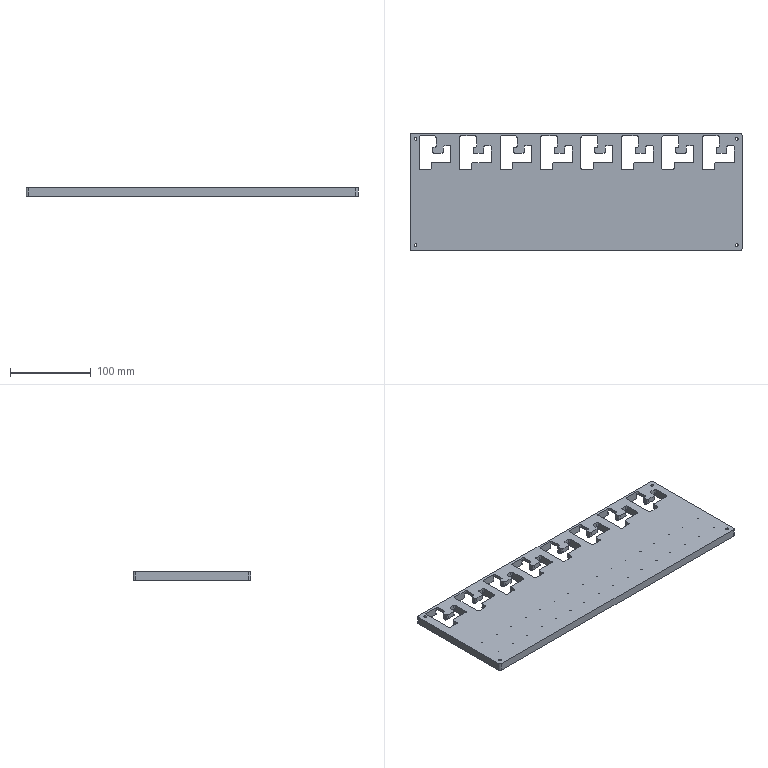NC program | NX | posted with a generic post | part box 410 x 145 x 10 mm
Lines 6396 to 7190 of 104733:
(CAVITY_MILL_COPY , TOOL : D6)
N12772 T06 M6
N12774 G54
N12776 G17 G0 G90 X-189.642 Y-62.962 S9500 M3
N12778 G43 Z30. H6
N12780 Z-0.5
N12782 G94 G1 X-190.342 Y-63.367 F1000.
N12784 G3 X-190.842 Y-64.233 R1.
N12786 G1 Y-65.086 F1650.
N12788 G2 X-191.001 Y-66.239 R4.25
N12790 G1 X-188.835
N12792 G3 X-187.969 Y-65.739 R1.
N12794 G1 X-187.565 Y-65.039
N12796 G0 X-189.642 Y-62.962 Z-1.
N12798 G1 X-190.342 Y-63.367 F1000.
N12800 G3 X-190.842 Y-64.233 R1.
N12802 G1 Y-65.086 F1650.
N12804 G2 X-191.001 Y-66.239 R4.25
N12806 G1 X-188.835
N12808 G3 X-187.969 Y-65.739 R1.
N12810 G1 X-187.565 Y-65.039
N12812 G0 X-189.642 Y-62.962 Z-1.5
N12814 G1 X-190.342 Y-63.367 F1000.
N12816 G3 X-190.842 Y-64.233 R1.
N12818 G1 Y-65.086 F1650.
N12820 G2 X-191.001 Y-66.239 R4.25
N12822 G1 X-188.835
N12824 G3 X-187.969 Y-65.739 R1.
N12826 G1 X-187.565 Y-65.039
N12828 G0 X-189.642 Y-62.962 Z-2.
N12830 G1 X-190.342 Y-63.367 F1000.
N12832 G3 X-190.842 Y-64.233 R1.
N12834 G1 Y-65.086 F1650.
N12836 G2 X-191.001 Y-66.239 R4.25
N12838 G1 X-188.835
N12840 G3 X-187.969 Y-65.739 R1.
N12842 G1 X-187.565 Y-65.039
N12844 G0 X-189.642 Y-62.962 Z-2.5
N12846 G1 X-190.342 Y-63.367 F1000.
N12848 G3 X-190.842 Y-64.233 R1.
N12850 G1 Y-65.086 F1650.
N12852 G2 X-191.001 Y-66.239 R4.25
N12854 G1 X-188.835
N12856 G3 X-187.969 Y-65.739 R1.
N12858 G1 X-187.565 Y-65.039
N12860 G0 X-189.642 Y-62.962 Z-3.
N12862 G1 X-190.342 Y-63.367 F1000.
N12864 G3 X-190.842 Y-64.233 R1.
N12866 G1 Y-65.086 F1650.
N12868 G2 X-191.001 Y-66.239 R4.25
N12870 G1 X-188.835
N12872 G3 X-187.969 Y-65.739 R1.
N12874 G1 X-187.565 Y-65.039
N12876 G0 X-189.642 Y-62.962 Z-3.5
N12878 G1 X-190.342 Y-63.367 F1000.
N12880 G3 X-190.842 Y-64.233 R1.
N12882 G1 Y-65.086 F1650.
N12884 G2 X-191.001 Y-66.239 R4.25
N12886 G1 X-188.835
N12888 G3 X-187.969 Y-65.739 R1.
N12890 G1 X-187.565 Y-65.039
N12892 G0 X-189.642 Y-62.962 Z-4.1
N12894 G1 X-190.342 Y-63.367 F1000.
N12896 G3 X-190.842 Y-64.233 R1.
N12898 G1 Y-65.086 F1650.
N12900 G2 X-191.001 Y-66.239 R4.25
N12902 G1 X-188.835
N12904 G3 X-187.969 Y-65.739 R1.
N12906 G1 X-187.565 Y-65.039
N12908 G0 X-189.642 Y-62.962 Z-4.575
N12910 G1 X-190.342 Y-63.367 F1000.
N12912 G3 X-190.842 Y-64.233 R1.
N12914 G1 Y-66.239 F1650.
N12916 X-188.835
N12918 G3 X-187.969 Y-65.739 R1.
N12920 G1 X-187.565 Y-65.039
N12922 G0 X-189.642 Y-62.962 Z-5.05
N12924 G1 X-190.342 Y-63.367 F1000.
N12926 G3 X-190.842 Y-64.233 R1.
N12928 G1 Y-66.239 F1650.
N12930 X-188.835
N12932 G3 X-187.969 Y-65.739 R1.
N12934 G1 X-187.565 Y-65.039
N12936 G0 X-189.642 Y-62.962 Z-5.525
N12938 G1 X-190.342 Y-63.367 F1000.
N12940 G3 X-190.842 Y-64.233 R1.
N12942 G1 Y-66.239 F1650.
N12944 X-188.835
N12946 G3 X-187.969 Y-65.739 R1.
N12948 G1 X-187.565 Y-65.039
N12950 G0 X-189.642 Y-62.962 Z-6.
N12952 G1 X-190.342 Y-63.367 F1000.
N12954 G3 X-190.842 Y-64.233 R1.
N12956 G1 Y-66.239 F1650.
N12958 X-188.835
N12960 G3 X-187.969 Y-65.739 R1.
N12962 G1 X-187.565 Y-65.039
N12964 G0 X-189.642 Y-62.962 Z-6.4
N12966 G1 X-190.342 Y-63.367 F1000.
N12968 G3 X-190.842 Y-64.233 R1.
N12970 G1 Y-66.239 F1650.
N12972 X-188.835
N12974 G3 X-187.969 Y-65.739 R1.
N12976 G1 X-187.565 Y-65.039
N12978 G0 X-189.642 Y-62.962 Z-6.933
N12980 G1 X-190.342 Y-63.367 F1000.
N12982 G3 X-190.842 Y-64.233 R1.
N12984 G1 Y-66.239 F1650.
N12986 X-188.835
N12988 G3 X-187.969 Y-65.739 R1.
N12990 G1 X-187.565 Y-65.039
N12992 G0 X-189.642 Y-62.962 Z-7.467
N12994 G1 X-190.342 Y-63.367 F1000.
N12996 G3 X-190.842 Y-64.233 R1.
N12998 G1 Y-66.239 F1650.
N13000 X-188.835
N13002 G3 X-187.969 Y-65.739 R1.
N13004 G1 X-187.565 Y-65.039
N13006 G0 X-189.642 Y-62.962 Z-8.
N13008 G1 X-190.342 Y-63.367 F1000.
N13010 G3 X-190.842 Y-64.233 R1.
N13012 G1 Y-66.239 F1650.
N13014 X-188.835
N13016 G3 X-187.969 Y-65.739 R1.
N13018 G1 X-187.565 Y-65.039
N13020 G0 X-189.642 Y-62.962 Z-8.5
N13022 G1 X-190.342 Y-63.367 F1000.
N13024 G3 X-190.842 Y-64.233 R1.
N13026 G1 Y-66.239 F1650.
N13028 X-188.835
N13030 G3 X-187.969 Y-65.739 R1.
N13032 G1 X-187.565 Y-65.039
N13034 G0 X-189.642 Y-62.962 Z-9.
N13036 G1 X-190.342 Y-63.367 F1000.
N13038 G3 X-190.842 Y-64.233 R1.
N13040 G1 Y-66.239 F1650.
N13042 X-188.835
N13044 G3 X-187.969 Y-65.739 R1.
N13046 G1 X-187.565 Y-65.039
N13048 G0 X-189.642 Y-62.962 Z-9.5
N13050 G1 X-190.342 Y-63.367 F1000.
N13052 G3 X-190.842 Y-64.233 R1.
N13054 G1 Y-66.239 F1650.
N13056 X-188.835
N13058 G3 X-187.969 Y-65.739 R1.
N13060 G1 X-187.565 Y-65.039
N13062 G0 X-189.642 Y-62.962 Z-10.
N13064 G1 X-190.342 Y-63.367 F1000.
N13066 G3 X-190.842 Y-64.233 R1.
N13068 G1 Y-66.239 F1650.
N13070 X-188.835
N13072 G3 X-187.969 Y-65.739 R1.
N13074 G1 X-187.565 Y-65.039
N13076 G0 Z30.
N13078 X-175.355 Y-60.831
N13080 Z-2.5
N13082 G1 X-175.051 Y-60.237 F1000.
N13084 G3 X-175.101 Y-59.238 R1.
N13086 G2 X-175.564 Y-58.315 R4.75 F1650.
N13088 G1 X-175.632 Y-58.313
N13090 X-175.759 Y-58.315
N13092 G2 X-176.59 Y-58.233 R4.25
N13094 G3 X-177.537 Y-58.554 R1.
N13096 G1 X-177.969 Y-59.047
N13098 G0 X-175.355 Y-60.831 Z-3.
N13100 G1 X-175.051 Y-60.237 F1000.
N13102 G3 X-175.101 Y-59.238 R1.
N13104 G2 X-175.564 Y-58.315 R4.75 F1650.
N13106 G1 X-175.632 Y-58.313
N13108 X-175.759 Y-58.315
N13110 G2 X-176.59 Y-58.233 R4.25
N13112 G3 X-177.537 Y-58.554 R1.
N13114 G1 X-177.97 Y-59.047
N13116 G0 X-175.355 Y-60.831 Z-3.5
N13118 G1 X-175.051 Y-60.237 F1000.
N13120 G3 X-175.101 Y-59.238 R1.
N13122 G2 X-175.564 Y-58.315 R4.75 F1650.
N13124 G1 X-175.632 Y-58.313
N13126 X-175.759 Y-58.315
N13128 G2 X-176.59 Y-58.233 R4.25
N13130 G3 X-177.537 Y-58.554 R1.
N13132 G1 X-177.97 Y-59.047
N13134 G0 X-175.355 Y-60.831 Z-4.1
N13136 G1 X-175.051 Y-60.237 F1000.
N13138 G3 X-175.101 Y-59.238 R1.
N13140 G2 X-175.564 Y-58.315 R4.75 F1650.
N13142 G1 X-175.632 Y-58.313
N13144 X-175.759 Y-58.315
N13146 G2 X-176.59 Y-58.233 R4.25
N13148 G3 X-177.538 Y-58.554 R1.
N13150 G1 X-177.97 Y-59.047
N13152 G0 X-175.355 Y-60.831 Z-4.575
N13154 G1 X-175.051 Y-60.237 F1000.
N13156 G3 X-175.101 Y-59.238 R1.
N13158 G2 X-175.564 Y-58.315 R4.75 F1650.
N13160 G1 X-175.632 Y-58.313
N13162 X-175.759 Y-58.315
N13164 G2 X-176.591 Y-58.233 R4.25
N13166 G3 X-177.538 Y-58.554 R1.
N13168 G1 X-177.97 Y-59.047
N13170 G0 X-175.355 Y-60.831 Z-5.05
N13172 G1 X-175.051 Y-60.237 F1000.
N13174 G3 X-175.101 Y-59.238 R1.
N13176 G2 X-175.564 Y-58.315 R4.75 F1650.
N13178 G1 X-175.632 Y-58.313
N13180 X-175.759 Y-58.315
N13182 G2 X-176.59 Y-58.233 R4.25
N13184 G3 X-177.537 Y-58.554 R1.
N13186 G1 X-177.97 Y-59.047
N13188 G0 X-175.355 Y-60.831 Z-5.525
N13190 G1 X-175.051 Y-60.237 F1000.
N13192 G3 X-175.101 Y-59.238 R1.
N13194 G2 X-175.564 Y-58.315 R4.75 F1650.
N13196 G1 X-175.632 Y-58.313
N13198 X-175.759 Y-58.315
N13200 G2 X-176.59 Y-58.233 R4.25
N13202 G3 X-177.537 Y-58.554 R1.
N13204 G1 X-177.97 Y-59.047
N13206 G0 X-175.355 Y-60.831 Z-6.
N13208 G1 X-175.05 Y-60.237 F1000.
N13210 G3 X-175.101 Y-59.238 R1.
N13212 G2 X-175.564 Y-58.315 R4.75 F1650.
N13214 G1 X-175.632 Y-58.313
N13216 X-175.759 Y-58.315
N13218 G2 X-176.59 Y-58.233 R4.25
N13220 G3 X-177.537 Y-58.554 R1.
N13222 G1 X-177.97 Y-59.047
N13224 G0 X-179.138 Y-65.039 Z-6.4
N13226 G1 X-178.734 Y-65.739 F1000.
N13228 G3 X-177.868 Y-66.239 R1.
N13230 G1 X-175.861 F1650.
N13232 Y-64.233
N13234 G3 X-176.361 Y-63.367 R1.
N13236 G1 X-177.061 Y-62.962
N13238 G0 X-179.138 Y-65.039 Z-6.933
N13240 G1 X-178.734 Y-65.739 F1000.
N13242 G3 X-177.868 Y-66.239 R1.
N13244 G1 X-175.861 F1650.
N13246 Y-64.233
N13248 G3 X-176.361 Y-63.367 R1.
N13250 G1 X-177.061 Y-62.962
N13252 G0 X-179.138 Y-65.039 Z-7.467
N13254 G1 X-178.734 Y-65.739 F1000.
N13256 G3 X-177.868 Y-66.239 R1.
N13258 G1 X-175.861 F1650.
N13260 Y-64.233
N13262 G3 X-176.361 Y-63.367 R1.
N13264 G1 X-177.061 Y-62.962
N13266 G0 X-179.138 Y-65.039 Z-8.
N13268 G1 X-178.734 Y-65.739 F1000.
N13270 G3 X-177.868 Y-66.239 R1.
N13272 G1 X-175.861 F1650.
N13274 Y-64.233
N13276 G3 X-176.361 Y-63.367 R1.
N13278 G1 X-177.061 Y-62.962
N13280 G0 X-179.138 Y-65.039 Z-8.5
N13282 G1 X-178.734 Y-65.739 F1000.
N13284 G3 X-177.868 Y-66.239 R1.
N13286 G1 X-175.861 F1650.
N13288 Y-64.233
N13290 G3 X-176.361 Y-63.367 R1.
N13292 G1 X-177.061 Y-62.962
N13294 G0 X-179.138 Y-65.039 Z-9.
N13296 G1 X-178.734 Y-65.739 F1000.
N13298 G3 X-177.868 Y-66.239 R1.
N13300 G1 X-175.861 F1650.
N13302 Y-64.233
N13304 G3 X-176.361 Y-63.367 R1.
N13306 G1 X-177.061 Y-62.962
N13308 G0 X-179.138 Y-65.039 Z-9.5
N13310 G1 X-178.734 Y-65.739 F1000.
N13312 G3 X-177.868 Y-66.239 R1.
N13314 G1 X-175.861 F1650.
N13316 Y-64.233
N13318 G3 X-176.361 Y-63.367 R1.
N13320 G1 X-177.061 Y-62.962
N13322 G0 X-179.138 Y-65.039 Z-10.
N13324 G1 X-178.734 Y-65.739 F1000.
N13326 G3 X-177.868 Y-66.239 R1.
N13328 G1 X-175.861 F1650.
N13330 Y-64.233
N13332 G3 X-176.361 Y-63.367 R1.
N13334 G1 X-177.061 Y-62.962
N13336 G0 Z30.
N13338 Y-61.228
N13340 Z-6.4
N13342 G1 X-176.361 Y-60.824 F1000.
N13344 G3 X-175.861 Y-59.958 R1.
N13346 G1 Y-58.314 F1650.
N13348 G2 X-177.276 Y-58.035 R4.25
N13350 G3 X-178.264 Y-58.193 R1.
N13352 G1 X-178.772 Y-58.607
N13354 G0 X-177.061 Y-61.228 Z-6.933
N13356 G1 X-176.361 Y-60.824 F1000.
N13358 G3 X-175.861 Y-59.958 R1.
N13360 G1 Y-58.314 F1650.
N13362 G2 X-177.276 Y-58.035 R4.25
N13364 G3 X-178.264 Y-58.193 R1.
N13366 G1 X-178.772 Y-58.607
N13368 G0 X-177.061 Y-61.228 Z-7.467
N13370 G1 X-176.361 Y-60.824 F1000.
N13372 G3 X-175.861 Y-59.958 R1.
N13374 G1 Y-58.314 F1650.
N13376 G2 X-177.276 Y-58.035 R4.25
N13378 G3 X-178.264 Y-58.193 R1.
N13380 G1 X-178.772 Y-58.607
N13382 G0 X-177.061 Y-61.228 Z-8.
N13384 G1 X-176.361 Y-60.824 F1000.
N13386 G3 X-175.861 Y-59.958 R1.
N13388 G1 Y-58.314 F1650.
N13390 G2 X-177.276 Y-58.035 R4.25
N13392 G3 X-178.264 Y-58.193 R1.
N13394 G1 X-178.772 Y-58.607
N13396 G0 X-177.061 Y-61.228 Z-8.5
N13398 G1 X-176.361 Y-60.824 F1000.
N13400 G3 X-175.861 Y-59.958 R1.
N13402 G1 Y-58.314 F1650.
N13404 G2 X-177.276 Y-58.035 R4.25
N13406 G3 X-178.264 Y-58.193 R1.
N13408 G1 X-178.772 Y-58.607
N13410 G0 X-177.061 Y-61.228 Z-9.
N13412 G1 X-176.361 Y-60.824 F1000.
N13414 G3 X-175.861 Y-59.958 R1.
N13416 G1 Y-58.314 F1650.
N13418 G2 X-177.276 Y-58.035 R4.25
N13420 G3 X-178.264 Y-58.193 R1.
N13422 G1 X-178.772 Y-58.607
N13424 G0 X-177.061 Y-61.228 Z-9.5
N13426 G1 X-176.361 Y-60.824 F1000.
N13428 G3 X-175.861 Y-59.958 R1.
N13430 G1 Y-58.314 F1650.
N13432 G2 X-177.276 Y-58.035 R4.25
N13434 G3 X-178.264 Y-58.193 R1.
N13436 G1 X-178.772 Y-58.607
N13438 G0 X-177.061 Y-61.228 Z-10.
N13440 G1 X-176.361 Y-60.824 F1000.
N13442 G3 X-175.861 Y-59.958 R1.
N13444 G1 Y-58.314 F1650.
N13446 G2 X-177.276 Y-58.035 R4.25
N13448 G3 X-178.264 Y-58.193 R1.
N13450 G1 X-178.772 Y-58.607
N13452 G0 Z30.
N13454 X-160.888 Y-45.752
N13456 Z-4.575
N13458 G1 X-161.232 Y-46.324 F1000.
N13460 G3 X-161.25 Y-47.323 R1.
N13462 G2 X-160.656 Y-49.623 R4.75 F1650.
N13464 G1 Y-54.394
N13466 X-157.442
N13468 Y-46.456
N13470 G3 X-157.942 Y-45.59 R1.
N13472 G1 X-158.642 Y-45.186
N13474 G0 X-160.888 Y-45.752 Z-5.05
N13476 G1 X-161.232 Y-46.324 F1000.
N13478 G3 X-161.25 Y-47.323 R1.
N13480 G2 X-160.656 Y-49.623 R4.75 F1650.
N13482 G1 Y-54.394
N13484 X-157.442
N13486 Y-46.456
N13488 G3 X-157.942 Y-45.59 R1.
N13490 G1 X-158.642 Y-45.186
N13492 G0 X-160.888 Y-45.752 Z-5.525
N13494 G1 X-161.232 Y-46.324 F1000.
N13496 G3 X-161.25 Y-47.323 R1.
N13498 G2 X-160.656 Y-49.623 R4.75 F1650.
N13500 G1 Y-54.394
N13502 X-157.442
N13504 Y-46.456
N13506 G3 X-157.942 Y-45.59 R1.
N13508 G1 X-158.642 Y-45.186
N13510 G0 X-160.888 Y-45.752 Z-6.
N13512 G1 X-161.232 Y-46.324 F1000.
N13514 G3 X-161.25 Y-47.323 R1.
N13516 G2 X-160.656 Y-49.623 R4.75 F1650.
N13518 G1 Y-54.394
N13520 X-157.442
N13522 Y-46.456
N13524 G3 X-157.942 Y-45.59 R1.
N13526 G1 X-158.642 Y-45.186
N13528 G0 X-160.888 Y-45.752 Z-6.4
N13530 G1 X-161.232 Y-46.324 F1000.
N13532 G3 X-161.25 Y-47.323 R1.
N13534 G2 X-160.656 Y-49.623 R4.75 F1650.
N13536 G1 Y-54.394
N13538 X-157.442
N13540 Y-46.456
N13542 G3 X-157.942 Y-45.59 R1.
N13544 G1 X-158.642 Y-45.186
N13546 G0 X-160.888 Y-45.752 Z-6.933
N13548 G1 X-161.232 Y-46.324 F1000.
N13550 G3 X-161.25 Y-47.323 R1.
N13552 G2 X-160.656 Y-49.623 R4.75 F1650.
N13554 G1 Y-54.394
N13556 X-157.442
N13558 Y-46.456
N13560 G3 X-157.942 Y-45.59 R1.
N13562 G1 X-158.642 Y-45.186
N13564 G0 X-160.888 Y-45.752 Z-7.467
N13566 G1 X-161.232 Y-46.324 F1000.
N13568 G3 X-161.25 Y-47.323 R1.
N13570 G2 X-160.656 Y-49.623 R4.75 F1650.
N13572 G1 Y-54.394
N13574 X-157.442
N13576 Y-46.456
N13578 G3 X-157.942 Y-45.59 R1.
N13580 G1 X-158.642 Y-45.186
N13582 G0 X-160.888 Y-45.752 Z-8.
N13584 G1 X-161.232 Y-46.324 F1000.
N13586 G3 X-161.25 Y-47.323 R1.
N13588 G2 X-160.656 Y-49.623 R4.75 F1650.
N13590 G1 Y-54.394
N13592 X-157.442
N13594 Y-46.456
N13596 G3 X-157.942 Y-45.59 R1.
N13598 G1 X-158.642 Y-45.186
N13600 G0 X-160.888 Y-45.752 Z-8.5
N13602 G1 X-161.232 Y-46.324 F1000.
N13604 G3 X-161.25 Y-47.323 R1.
N13606 G2 X-160.656 Y-49.623 R4.75 F1650.
N13608 G1 Y-54.394
N13610 X-157.442
N13612 Y-46.456
N13614 G3 X-157.942 Y-45.59 R1.
N13616 G1 X-158.642 Y-45.186
N13618 G0 X-160.888 Y-45.752 Z-9.
N13620 G1 X-161.232 Y-46.324 F1000.
N13622 G3 X-161.25 Y-47.323 R1.
N13624 G2 X-160.656 Y-49.623 R4.75 F1650.
N13626 G1 Y-54.394
N13628 X-157.442
N13630 Y-46.456
N13632 G3 X-157.942 Y-45.59 R1.
N13634 G1 X-158.642 Y-45.186
N13636 G0 X-160.888 Y-45.752 Z-9.5
N13638 G1 X-161.232 Y-46.324 F1000.
N13640 G3 X-161.25 Y-47.323 R1.
N13642 G2 X-160.656 Y-49.623 R4.75 F1650.
N13644 G1 Y-54.394
N13646 X-157.442
N13648 Y-46.456
N13650 G3 X-157.942 Y-45.59 R1.
N13652 G1 X-158.642 Y-45.186
N13654 G0 X-160.888 Y-45.752 Z-10.
N13656 G1 X-161.232 Y-46.324 F1000.
N13658 G3 X-161.25 Y-47.323 R1.
N13660 G2 X-160.656 Y-49.623 R4.75 F1650.
N13662 G1 Y-54.394
N13664 X-157.442
N13666 Y-46.456
N13668 G3 X-157.942 Y-45.59 R1.
N13670 G1 X-158.642 Y-45.186
N13672 G0 Z30.
N13674 X-160.294 Y-66.106
N13676 Z-0.5
N13678 G1 X-159.759 Y-66.505 F1000.
N13680 G3 X-158.766 Y-66.623 R1.
N13682 G2 X-157.278 Y-66.255 R4.75 F1650.
N13684 X-157.442 Y-65.086 R4.25
N13686 G1 Y-64.723
N13688 G3 X-157.942 Y-63.857 R1.
N13690 G1 X-158.642 Y-63.452
N13692 G0 X-160.294 Y-66.106 Z-1.
N13694 G1 X-159.759 Y-66.505 F1000.
N13696 G3 X-158.766 Y-66.623 R1.
N13698 G2 X-157.278 Y-66.255 R4.75 F1650.
N13700 X-157.442 Y-65.086 R4.25
N13702 G1 Y-64.723
N13704 G3 X-157.942 Y-63.857 R1.
N13706 G1 X-158.642 Y-63.452
N13708 G0 X-160.294 Y-66.106 Z-1.5
N13710 G1 X-159.759 Y-66.505 F1000.
N13712 G3 X-158.766 Y-66.623 R1.
N13714 G2 X-157.278 Y-66.255 R4.75 F1650.
N13716 X-157.442 Y-65.086 R4.25
N13718 G1 Y-64.723
N13720 G3 X-157.942 Y-63.857 R1.
N13722 G1 X-158.642 Y-63.452
N13724 G0 X-160.294 Y-66.106 Z-2.
N13726 G1 X-159.759 Y-66.505 F1000.
N13728 G3 X-158.766 Y-66.623 R1.
N13730 G2 X-157.278 Y-66.255 R4.75 F1650.
N13732 X-157.442 Y-65.086 R4.25
N13734 G1 Y-64.723
N13736 G3 X-157.942 Y-63.857 R1.
N13738 G1 X-158.642 Y-63.452
N13740 G0 X-160.294 Y-66.106 Z-2.5
N13742 G1 X-159.759 Y-66.505 F1000.
N13744 G3 X-158.766 Y-66.623 R1.
N13746 G2 X-157.278 Y-66.255 R4.75 F1650.
N13748 X-157.442 Y-65.086 R4.25
N13750 G1 Y-64.723
N13752 G3 X-157.942 Y-63.857 R1.
N13754 G1 X-158.642 Y-63.452
N13756 G0 X-160.294 Y-66.106 Z-3.
N13758 G1 X-159.759 Y-66.505 F1000.
N13760 G3 X-158.766 Y-66.623 R1.
N13762 G2 X-157.278 Y-66.255 R4.75 F1650.
N13764 X-157.442 Y-65.086 R4.25
N13766 G1 Y-64.723
N13768 G3 X-157.942 Y-63.857 R1.
N13770 G1 X-158.642 Y-63.452
N13772 G0 X-160.294 Y-66.106 Z-3.5
N13774 G1 X-159.759 Y-66.505 F1000.
N13776 G3 X-158.766 Y-66.623 R1.
N13778 G2 X-157.278 Y-66.255 R4.75 F1650.
N13780 X-157.442 Y-65.086 R4.25
N13782 G1 Y-64.723
N13784 G3 X-157.942 Y-63.857 R1.
N13786 G1 X-158.642 Y-63.452
N13788 G0 X-160.294 Y-66.106 Z-4.1
N13790 G1 X-159.759 Y-66.505 F1000.
N13792 G3 X-158.766 Y-66.623 R1.
N13794 G2 X-157.278 Y-66.255 R4.75 F1650.
N13796 X-157.442 Y-65.086 R4.25
N13798 G1 Y-64.723
N13800 G3 X-157.942 Y-63.857 R1.
N13802 G1 X-158.642 Y-63.452
N13804 G0 Z30.
N13806 X-162.844 Y-64.687
N13808 Z-4.575
N13810 G1 X-162.144 Y-64.283 F1000.
N13812 G3 X-161.644 Y-63.416 R1.
N13814 G1 Y-61.41 F1650.
N13816 X-163.651
N13818 G3 X-164.517 Y-61.91 R1.
N13820 G1 X-164.921 Y-62.61
N13822 G0 X-162.844 Y-64.687 Z-5.05
N13824 G1 X-162.144 Y-64.283 F1000.
N13826 G3 X-161.644 Y-63.416 R1.
N13828 G1 Y-61.41 F1650.
N13830 X-163.651
N13832 G3 X-164.517 Y-61.91 R1.
N13834 G1 X-164.921 Y-62.61
N13836 G0 X-162.844 Y-64.687 Z-5.525
N13838 G1 X-162.144 Y-64.283 F1000.
N13840 G3 X-161.644 Y-63.416 R1.
N13842 G1 Y-61.41 F1650.
N13844 X-163.651
N13846 G3 X-164.517 Y-61.91 R1.
N13848 G1 X-164.921 Y-62.61
N13850 G0 X-162.844 Y-64.687 Z-6.
N13852 G1 X-162.144 Y-64.283 F1000.
N13854 G3 X-161.644 Y-63.416 R1.
N13856 G1 Y-61.41 F1650.
N13858 X-163.651
N13860 G3 X-164.517 Y-61.91 R1.
N13862 G1 X-164.921 Y-62.61
N13864 G0 Z30.
N13866 X-139.642 Y-62.962
N13868 Z-0.5
N13870 G1 X-140.342 Y-63.367 F1000.
N13872 G3 X-140.842 Y-64.233 R1.
N13874 G1 Y-65.086 F1650.
N13876 G2 X-141.001 Y-66.239 R4.25
N13878 G1 X-138.835
N13880 G3 X-137.969 Y-65.739 R1.
N13882 G1 X-137.565 Y-65.039
N13884 G0 X-139.642 Y-62.962 Z-1.
N13886 G1 X-140.342 Y-63.367 F1000.
N13888 G3 X-140.842 Y-64.233 R1.
N13890 G1 Y-65.086 F1650.
N13892 G2 X-141.001 Y-66.239 R4.25
N13894 G1 X-138.835
N13896 G3 X-137.969 Y-65.739 R1.
N13898 G1 X-137.565 Y-65.039
N13900 G0 X-139.642 Y-62.962 Z-1.5
N13902 G1 X-140.342 Y-63.367 F1000.
N13904 G3 X-140.842 Y-64.233 R1.
N13906 G1 Y-65.086 F1650.
N13908 G2 X-141.001 Y-66.239 R4.25
N13910 G1 X-138.835
N13912 G3 X-137.969 Y-65.739 R1.
N13914 G1 X-137.565 Y-65.039
N13916 G0 X-139.642 Y-62.962 Z-2.
N13918 G1 X-140.342 Y-63.367 F1000.
N13920 G3 X-140.842 Y-64.233 R1.
N13922 G1 Y-65.086 F1650.
N13924 G2 X-141.001 Y-66.239 R4.25
N13926 G1 X-138.835
N13928 G3 X-137.969 Y-65.739 R1.
N13930 G1 X-137.565 Y-65.039
N13932 G0 X-139.642 Y-62.962 Z-2.5
N13934 G1 X-140.342 Y-63.367 F1000.
N13936 G3 X-140.842 Y-64.233 R1.
N13938 G1 Y-65.086 F1650.
N13940 G2 X-141.001 Y-66.239 R4.25
N13942 G1 X-138.835
N13944 G3 X-137.969 Y-65.739 R1.
N13946 G1 X-137.565 Y-65.039
N13948 G0 X-139.642 Y-62.962 Z-3.
N13950 G1 X-140.342 Y-63.367 F1000.
N13952 G3 X-140.842 Y-64.233 R1.
N13954 G1 Y-65.086 F1650.
N13956 G2 X-141.001 Y-66.239 R4.25
N13958 G1 X-138.835
N13960 G3 X-137.969 Y-65.739 R1.
N13962 G1 X-137.565 Y-65.039
N13964 G0 X-139.642 Y-62.962 Z-3.5
N13966 G1 X-140.342 Y-63.367 F1000.
N13968 G3 X-140.842 Y-64.233 R1.
N13970 G1 Y-65.086 F1650.
N13972 G2 X-141.001 Y-66.239 R4.25
N13974 G1 X-138.835
N13976 G3 X-137.969 Y-65.739 R1.
N13978 G1 X-137.565 Y-65.039
N13980 G0 X-139.642 Y-62.962 Z-4.1
N13982 G1 X-140.342 Y-63.367 F1000.
N13984 G3 X-140.842 Y-64.233 R1.
N13986 G1 Y-65.086 F1650.
N13988 G2 X-141.001 Y-66.239 R4.25
N13990 G1 X-138.835
N13992 G3 X-137.969 Y-65.739 R1.
N13994 G1 X-137.565 Y-65.039
N13996 G0 X-139.642 Y-62.962 Z-4.575
N13998 G1 X-140.342 Y-63.367 F1000.
N14000 G3 X-140.842 Y-64.233 R1.
N14002 G1 Y-66.239 F1650.
N14004 X-138.835
N14006 G3 X-137.969 Y-65.739 R1.
N14008 G1 X-137.565 Y-65.039
N14010 G0 X-139.642 Y-62.962 Z-5.05
N14012 G1 X-140.342 Y-63.367 F1000.
N14014 G3 X-140.842 Y-64.233 R1.
N14016 G1 Y-66.239 F1650.
N14018 X-138.835
N14020 G3 X-137.969 Y-65.739 R1.
N14022 G1 X-137.565 Y-65.039
N14024 G0 X-139.642 Y-62.962 Z-5.525
N14026 G1 X-140.342 Y-63.367 F1000.
N14028 G3 X-140.842 Y-64.233 R1.
N14030 G1 Y-66.239 F1650.
N14032 X-138.835
N14034 G3 X-137.969 Y-65.739 R1.
N14036 G1 X-137.565 Y-65.039
N14038 G0 X-139.642 Y-62.962 Z-6.
N14040 G1 X-140.342 Y-63.367 F1000.
N14042 G3 X-140.842 Y-64.233 R1.
N14044 G1 Y-66.239 F1650.
N14046 X-138.835
N14048 G3 X-137.969 Y-65.739 R1.
N14050 G1 X-137.565 Y-65.039
N14052 G0 X-139.642 Y-62.962 Z-6.4
N14054 G1 X-140.342 Y-63.367 F1000.
N14056 G3 X-140.842 Y-64.233 R1.
N14058 G1 Y-66.239 F1650.
N14060 X-138.835
N14062 G3 X-137.969 Y-65.739 R1.
N14064 G1 X-137.565 Y-65.039
N14066 G0 X-139.642 Y-62.962 Z-6.933
N14068 G1 X-140.342 Y-63.367 F1000.
N14070 G3 X-140.842 Y-64.233 R1.
N14072 G1 Y-66.239 F1650.
N14074 X-138.835
N14076 G3 X-137.969 Y-65.739 R1.
N14078 G1 X-137.565 Y-65.039
N14080 G0 X-139.642 Y-62.962 Z-7.467
N14082 G1 X-140.342 Y-63.367 F1000.
N14084 G3 X-140.842 Y-64.233 R1.
N14086 G1 Y-66.239 F1650.
N14088 X-138.835
N14090 G3 X-137.969 Y-65.739 R1.
N14092 G1 X-137.565 Y-65.039
N14094 G0 X-139.642 Y-62.962 Z-8.
N14096 G1 X-140.342 Y-63.367 F1000.
N14098 G3 X-140.842 Y-64.233 R1.
N14100 G1 Y-66.239 F1650.
N14102 X-138.835
N14104 G3 X-137.969 Y-65.739 R1.
N14106 G1 X-137.565 Y-65.039
N14108 G0 X-139.642 Y-62.962 Z-8.5
N14110 G1 X-140.342 Y-63.367 F1000.
N14112 G3 X-140.842 Y-64.233 R1.
N14114 G1 Y-66.239 F1650.
N14116 X-138.835
N14118 G3 X-137.969 Y-65.739 R1.
N14120 G1 X-137.565 Y-65.039
N14122 G0 X-139.642 Y-62.962 Z-9.
N14124 G1 X-140.342 Y-63.367 F1000.
N14126 G3 X-140.842 Y-64.233 R1.
N14128 G1 Y-66.239 F1650.
N14130 X-138.835
N14132 G3 X-137.969 Y-65.739 R1.
N14134 G1 X-137.565 Y-65.039
N14136 G0 X-139.642 Y-62.962 Z-9.5
N14138 G1 X-140.342 Y-63.367 F1000.
N14140 G3 X-140.842 Y-64.233 R1.
N14142 G1 Y-66.239 F1650.
N14144 X-138.835
N14146 G3 X-137.969 Y-65.739 R1.
N14148 G1 X-137.565 Y-65.039
N14150 G0 X-139.642 Y-62.962 Z-10.
N14152 G1 X-140.342 Y-63.367 F1000.
N14154 G3 X-140.842 Y-64.233 R1.
N14156 G1 Y-66.239 F1650.
N14158 X-138.835
N14160 G3 X-137.969 Y-65.739 R1.
N14162 G1 X-137.565 Y-65.039
N14164 G0 Z30.
N14166 X-110.283 Y-66.098
N14168 Z-0.5
N14170 G1 X-109.749 Y-66.499 F1000.
N14172 G3 X-108.757 Y-66.619 R1.
N14174 G2 X-107.373 Y-66.263 R4.75 F1650.
N14176 G1 X-107.277 Y-66.257
N14178 G2 X-107.442 Y-65.086 R4.25
N14180 G1 Y-64.726
N14182 G3 X-107.942 Y-63.86 R1.
N14184 G1 X-108.642 Y-63.456
N14186 G0 X-110.285 Y-66.1 Z-1.
N14188 G1 X-109.751 Y-66.5 F1000.
N14190 G3 X-108.759 Y-66.62 R1.
N14192 G2 X-107.373 Y-66.263 R4.75 F1650.
N14194 G1 X-107.277 Y-66.257
N14196 G2 X-107.442 Y-65.086 R4.25
N14198 G1 Y-64.725
N14200 G3 X-107.942 Y-63.859 R1.
N14202 G1 X-108.642 Y-63.455
N14204 G0 X-110.287 Y-66.101 Z-1.5
N14206 G1 X-109.753 Y-66.501 F1000.
N14208 G3 X-108.761 Y-66.621 R1.
N14210 G2 X-107.373 Y-66.263 R4.75 F1650.
N14212 G1 X-107.277 Y-66.256
N14214 G2 X-107.442 Y-65.086 R4.25
N14216 G1 Y-64.725
N14218 G3 X-107.942 Y-63.858 R1.
N14220 G1 X-108.642 Y-63.454
N14222 G0 X-110.289 Y-66.103 Z-2.
N14224 G1 X-109.755 Y-66.503 F1000.
N14226 G3 X-108.762 Y-66.622 R1.
N14228 G2 X-107.373 Y-66.263 R4.75 F1650.
N14230 G1 X-107.277 Y-66.256
N14232 G2 X-107.442 Y-65.086 R4.25
N14234 G1 Y-64.724
N14236 G3 X-107.942 Y-63.858 R1.
N14238 G1 X-108.642 Y-63.454
N14240 G0 X-110.291 Y-66.104 Z-2.5
N14242 G1 X-109.757 Y-66.504 F1000.
N14244 G3 X-108.764 Y-66.623 R1.
N14246 G2 X-107.373 Y-66.263 R4.75 F1650.
N14248 G1 X-107.278 Y-66.255
N14250 G2 X-107.442 Y-65.086 R4.25
N14252 G1 Y-64.723
N14254 G3 X-107.942 Y-63.857 R1.
N14256 G1 X-108.642 Y-63.453
N14258 G0 X-110.294 Y-66.106 Z-3.
N14260 G1 X-109.759 Y-66.505 F1000.
N14262 G3 X-108.766 Y-66.623 R1.
N14264 G2 X-107.373 Y-66.263 R4.75 F1650.
N14266 G1 X-107.278 Y-66.253
N14268 G2 X-107.442 Y-65.086 R4.25
N14270 G1 Y-64.723
N14272 G3 X-107.942 Y-63.857 R1.
N14274 G1 X-108.642 Y-63.452
N14276 G0 X-110.296 Y-66.107 Z-3.5
N14278 G1 X-109.761 Y-66.507 F1000.
N14280 G3 X-108.768 Y-66.624 R1.
N14282 G2 X-107.278 Y-66.253 R4.752 F1650.
N14284 X-107.442 Y-65.086 R4.25
N14286 G1 Y-64.722
N14288 G3 X-107.942 Y-63.856 R1.
N14290 G1 X-108.642 Y-63.452
N14292 G0 X-110.298 Y-66.109 Z-4.1
N14294 G1 X-109.764 Y-66.508 F1000.
N14296 G3 X-108.771 Y-66.625 R1.
N14298 G2 X-107.278 Y-66.253 R4.752 F1650.
N14300 X-107.442 Y-65.086 R4.25
N14302 G1 Y-64.721
N14304 G3 X-107.942 Y-63.855 R1.
N14306 G1 X-108.642 Y-63.451
N14308 G0 Z30.
N14310 X-112.844 Y-64.687
N14312 Z-4.575
N14314 G1 X-112.144 Y-64.283 F1000.
N14316 G3 X-111.644 Y-63.417 R1.
N14318 G1 Y-61.41 F1650.
N14320 X-113.651
N14322 G3 X-114.517 Y-61.91 R1.
N14324 G1 X-114.921 Y-62.61
N14326 G0 X-112.844 Y-64.687 Z-5.05
N14328 G1 X-112.144 Y-64.283 F1000.
N14330 G3 X-111.644 Y-63.417 R1.
N14332 G1 Y-61.41 F1650.
N14334 X-113.651
N14336 G3 X-114.517 Y-61.91 R1.
N14338 G1 X-114.921 Y-62.61
N14340 G0 X-112.844 Y-64.687 Z-5.525
N14342 G1 X-112.144 Y-64.283 F1000.
N14344 G3 X-111.644 Y-63.417 R1.
N14346 G1 Y-61.41 F1650.
N14348 X-113.651
N14350 G3 X-114.517 Y-61.91 R1.
N14352 G1 X-114.921 Y-62.61
N14354 G0 X-112.844 Y-64.687 Z-6.